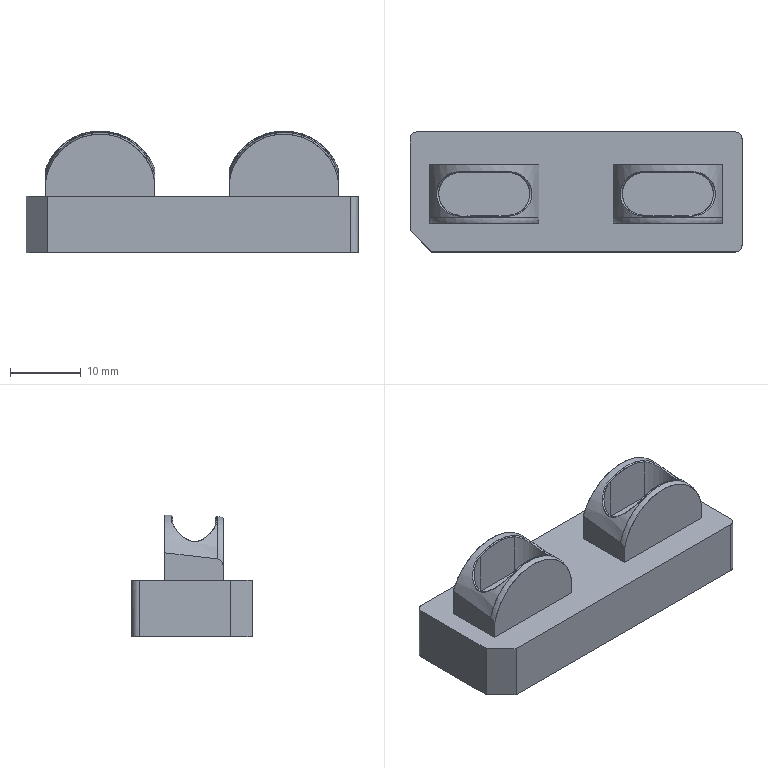NC program | PowerMill | posted with a generic post | part box 47 x 17 x 17.251 mm
Lines 1 to 1041 of 158620:
%
O0001
N104 ( POWERMILL CB  : 2026004.0)
N105 ( POST VER      : 2026.0.0.5161)
N106 ( OPTION FILE   : FANUC)
N107 ( OUTPUT WORKPLANE : WORLD)
N108 (  )
N109 ( TOOL LIST )
N110 (---------------------------------------)
N111 ( NO. | ID        | DIA.| TIP RAD|LENGTH)
N112 (---------------------------------------)
N113 (    1|D10C_1_1   |10.0 |  0.0   |72.72 )
N114 (   15|D3C_1_1    | 3.0 |  0.0   |64.44 )
N115 (    3|D10_1_1    |10.0 |  0.0   | 72.4 )
N116 (   22|R1.5_1_1   | 3.0 |  1.5   |63.12 )
N117 (   10|D3_1_1     | 3.0 |  0.0   |62.36 )
N118 (   13|TEXT_D4_1_1| 4.0 |  0.3   |64.52 )
N119 (---------------------------------------)
N120 (  )
N121 ( NUMBER OF TOOLPATHS: 11.0 )
N122 ( ESTIMATED PROGRAM DURATION: 0 HOURS 14 MIN 53 SEC)
N123 (  )
N124 G00 G21 G80 G40 G17
N125 G90
N126 G54
N127 G53 Z0.0
N128 (---------------)
N129 ( START TOOLPATH : 精公开粗01-扫面平行-D10C )
N130 (---------------)
N131 ( TOOL NO.    :1 )
N132 ( TOOL TYPE   : ENDMILL)
N133 ( TOOL ID     : D10C_1_1)
N134 ( TOOL DIA    : 10.0 LENGTH 72.72)
N135 T1
N136 M6
N137 S8000 M03
N138 G00 G90 X0.0 Y0.0
N139 G43 Z10.2 H1
N140
N141 G05 P10000 R4
N142 X31.28 Y11.28
N143 Z1.128
N144 G01 Z-0.072 F6000.0
N145 X26.28 F10000.0
N146 X-26.28
N147 Y5.64
N148 X26.28
N149 Y0.0
N150 X-26.28
N151 Y-5.64
N152 X26.28
N153 Y-11.28
N154 X-26.28
N155 X-31.28
N156 G00 Z10.2
N157 G05 P0
N158 (---------------)
N159 ( END TOOLPATH : 精公开粗01-扫面平行-D10C )
N160 (---------------)
N161 ( START TOOLPATH : 精公开粗01-外形偏置-D10C )
N162 (---------------)
N163 G00 X0.0 Y-0.283 Z9.878
N164 G05 P10000 R4
N165 X-17.5054 Y16.91
N166 Z0.6807
N167 G01 Z-0.5193 F6000.0
N168 Y16.3825 F10000.0
N169 G03 X-12.7579 Y11.635 I4.7475 J0.0
N170 G01 X12.758
N171 X12.7615 Y9.1322
N172 X15.0818 Y9.1355
N173 X15.8552 Y9.1085
N174 X16.5574 Y8.9981
N175 X17.4021 Y8.7405
N176 X18.1755 Y8.3597
N177 X18.393 Y8.2247
N178 X18.9489 Y7.8001
N179 X19.3124 Y7.4513
N180 X19.7224 Y6.9589
N181 X19.9196 Y6.6778
N182 X20.3286 Y5.9044
N183 X20.589 Y5.131
N184 X20.7229 Y4.3576
N185 X20.74 Y3.5841
N186 X20.657 Y2.8107
N187 X20.5342 Y2.0373
N188 X20.3467 Y1.2639
N189 X20.0249 Y0.4904
N190 X19.7224 Y-0.0237
N191 X19.5378 Y-0.283
N192 X19.22 Y-0.663
N193 G03 X19.1311 Y-1.2001 I0.3693 J-0.337
N194 G01 X19.4061 Y-1.8299
N195 X19.594 Y-2.6033
N196 X19.6618 Y-3.3767
N197 X19.6278 Y-4.1501
N198 X19.489 Y-4.9236
N199 X19.2244 Y-5.697
N200 X18.8199 Y-6.4704
N201 X18.2841 Y-7.2438
N202 X17.4821 Y-8.0173
N203 X16.6287 Y-8.6151
N204 X16.2904 Y-8.7907
N205 X15.8552 Y-8.9797
N206 X15.0818 Y-9.2292
N207 X14.3084 Y-9.4135
N208 X13.535 Y-9.5002
N209 X12.7615 Y-9.5116
N210 X11.9881 Y-9.4606
N211 X11.2147 Y-9.3047
N212 X10.4413 Y-9.0907
N213 X9.6678 Y-8.7734
N214 X8.8944 Y-8.3039
N215 X8.5171 Y-8.0173
N216 X8.121 Y-7.67
N217 X7.7159 Y-7.2438
N218 X7.3476 Y-6.7404
N219 X7.1809 Y-6.4704
N220 X6.7756 Y-5.697
N221 X6.5144 Y-4.9236
N222 X6.3722 Y-4.1501
N223 X6.3404 Y-3.3767
N224 X6.406 Y-2.6033
N225 X6.5939 Y-1.8299
N226 X6.8758 Y-1.1862
N227 G03 X6.7915 Y-0.6534 I-0.4579 J0.2006
N228 G01 X6.4622 Y-0.283
N229 X5.9751 Y0.4904
N230 X5.6533 Y1.2639
N231 X5.4678 Y2.0373
N232 X5.2617 Y3.5841
N233 X5.2771 Y4.3576
N234 X5.411 Y5.131
N235 X5.6731 Y5.9044
N236 X6.0812 Y6.6778
N237 X6.6856 Y7.4513
N238 X7.3476 Y8.0401
N239 X7.6061 Y8.2247
N240 X8.121 Y8.5254
N241 X8.8944 Y8.8474
N242 X9.4406 Y8.9981
N243 X10.4413 Y9.1289
N244 X12.7615 Y9.1322
N245 X12.758 Y11.635
N246 X27.507
N247 G02 X28.507 Y10.635 I0.0 J-1.0
N248 G01 Y-11.201
N249 G02 X27.507 Y-12.201 I-1.0 J0.0
N250 G01 X-27.507
N251 G02 X-28.507 Y-11.201 I0.0 J1.0
N252 G01 Y10.635
N253 G02 X-27.507 Y11.635 I1.0 J0.0
N254 G01 X-12.7579
N255 X-12.7615 Y9.1322
N256 X-10.4413 Y9.1288
N257 X-9.6678 Y9.0428
N258 X-8.8944 Y8.8473
N259 X-8.121 Y8.5254
N260 X-7.6061 Y8.2247
N261 X-7.3476 Y8.0401
N262 X-6.6856 Y7.4513
N263 X-6.0804 Y6.6778
N264 X-5.6713 Y5.9044
N265 X-5.411 Y5.131
N266 X-0.0017 Y6.1258
N267 X-0.0034 Y6.135
N268 X0.0034
N269 X0.0 Y6.1165
N270 X-0.0017 Y6.1258
N271 X-5.411 Y5.131
N272 X-5.2771 Y4.3576
N273 X-5.2608 Y3.5841
N274 X-5.3417 Y2.8107
N275 X-5.4657 Y2.0373
N276 X-5.6533 Y1.2639
N277 X-5.9751 Y0.4904
N278 X-6.4622 Y-0.283
N279 X-6.7824 Y-0.6429
N280 G03 X-6.8707 Y-1.1667 I0.3736 J-0.3323
N281 G01 X-6.5959 Y-1.8299
N282 X-6.406 Y-2.6033
N283 X-6.3433 Y-3.3392
N284 X-1.2755 Y-3.4159
N285 X-1.2507 Y-1.7746
N286 G02 X1.2556 Y-1.7764 I1.2532 J-0.019
N287 G01 X1.2811 Y-3.6293
N288 X1.3082 Y-4.2623
N289 X1.372 Y-4.8926
N290 X1.4318 Y-5.3509
N291 G02 X0.2456 Y-6.7289 I-1.2099 J-0.158
N292 G01 X-0.1982 Y-6.7375
N293 G02 X-1.431 Y-5.3585 I-0.0237 J1.2194
N294 G01 X-1.3708 Y-4.9021
N295 X-1.3067 Y-4.2776
N296 X-1.279 Y-3.6503
N297 X-1.2755 Y-3.4159
N298 X-6.3433 Y-3.3392
N299 X-6.3401 Y-3.3767
N300 X-6.3722 Y-4.1501
N301 X-6.5114 Y-4.9236
N302 X-6.7756 Y-5.697
N303 X-7.3476 Y-6.7404
N304 X-7.7213 Y-7.2438
N305 X-8.121 Y-7.67
N306 X-8.5201 Y-8.0173
N307 X-8.8944 Y-8.3039
N308 X-9.7111 Y-8.7907
N309 X-10.4413 Y-9.0907
N310 X-11.2147 Y-9.307
N311 X-11.9881 Y-9.4606
N312 X-12.7615 Y-9.5073
N313 X-13.535 Y-9.5014
N314 X-14.3084 Y-9.4135
N315 X-15.0818 Y-9.2292
N316 X-15.8552 Y-8.9797
N317 X-16.6287 Y-8.6151
N318 X-17.4813 Y-8.0173
N319 X-18.2841 Y-7.2438
N320 X-18.8183 Y-6.4704
N321 X-19.2244 Y-5.697
N322 X-19.4849 Y-4.9236
N323 X-19.6278 Y-4.1501
N324 X-19.6618 Y-3.3767
N325 X-19.594 Y-2.6033
N326 X-19.4061 Y-1.8299
N327 X-19.1308 Y-1.2012
N328 G03 X-19.2193 Y-0.6637 I-0.4579 J0.2006
N329 G01 X-19.7224 Y-0.0237
N330 X-20.0249 Y0.4904
N331 X-20.3467 Y1.2639
N332 X-20.4958 Y1.836
N333 X-20.7387 Y3.5841
N334 X-20.7229 Y4.3576
N335 X-20.5886 Y5.131
N336 X-20.3287 Y5.9044
N337 X-19.9196 Y6.6778
N338 X-19.7224 Y6.9585
N339 X-19.3142 Y7.4513
N340 X-18.9489 Y7.8001
N341 X-18.3932 Y8.2247
N342 X-18.1755 Y8.3596
N343 X-17.4021 Y8.7406
N344 X-16.6287 Y8.9813
N345 X-15.8552 Y9.1076
N346 X-15.0818 Y9.1355
N347 X-12.7615 Y9.1322
N348 X-12.7579 Y11.635
N349 G00 Z3.2834
N350 G01 X-17.5054 Y16.91
N351 G00 Z0.2834
N352 G01 Z-0.9166 F6000.0
N353 Y16.3825 F10000.0
N354 G03 X-12.7579 Y11.635 I4.7475 J0.0
N355 G01 X12.7615
N356 Y9.1356
N357 X15.8552
N358 X16.6287 Y9.1286
N359 X17.4021 Y9.0388
N360 X18.1755 Y8.8346
N361 X18.9489 Y8.4994
N362 X19.4118 Y8.2247
N363 X19.7224 Y7.9996
N364 X20.3275 Y7.4513
N365 X20.4958 Y7.2629
N366 X20.9306 Y6.6778
N367 X21.2692 Y6.053
N368 X21.598 Y5.131
N369 X21.7316 Y4.3576
N370 X21.7486 Y3.5841
N371 X21.6031 Y2.0373
N372 X21.4153 Y1.2639
N373 X21.2692 Y0.8725
N374 X21.0944 Y0.4904
N375 X20.6089 Y-0.283
N376 X20.5103 Y-0.4012
N377 G03 X20.4588 Y-0.9675 I0.3838 J-0.3204
N378 G01 X20.509 Y-1.0564
N379 X20.8302 Y-1.8299
N380 X21.0174 Y-2.6033
N381 X21.0885 Y-3.3767
N382 X21.0627 Y-4.1501
N383 X20.9277 Y-4.9236
N384 X20.6786 Y-5.697
N385 X20.3215 Y-6.4704
N386 X19.7224 Y-7.3692
N387 X18.9489 Y-8.1895
N388 X18.1887 Y-8.7907
N389 X17.4021 Y-9.2212
N390 X16.6287 Y-9.495
N391 X16.3488 Y-9.5641
N392 X15.8552 Y-9.6494
N393 X15.0818 Y-9.7019
N394 X11.2147 Y-9.702
N395 X10.4413 Y-9.6799
N396 X9.6501 Y-9.5641
N397 X8.8944 Y-9.3411
N398 X8.121 Y-8.9802
N399 X7.8138 Y-8.7907
N400 X7.3476 Y-8.4482
N401 X6.5741 Y-7.7184
N402 X6.1816 Y-7.2438
N403 X5.6785 Y-6.4704
N404 X5.3209 Y-5.697
N405 X5.0726 Y-4.9236
N406 X4.9365 Y-4.1501
N407 X4.9139 Y-3.3767
N408 X4.9804 Y-2.6274
N409 X0.4981 Y-2.2296
N410 X4.9804 Y-2.6274
N411 X4.9826 Y-2.6033
N412 X5.1699 Y-1.8299
N413 X5.491 Y-1.0564
N414 X5.5409 Y-0.9685
N415 G03 X5.4902 Y-0.4016 I-0.4348 J0.2468
N416 G01 X5.3913 Y-0.283
N417 X4.9056 Y0.4904
N418 X4.5841 Y1.2639
N419 X4.3969 Y2.0373
N420 X4.2538 Y3.5548
N421 Y4.166
N422 X4.4022 Y5.131
N423 X4.6628 Y5.9044
N424 X5.0273 Y6.6094
N425 X5.6719 Y7.4513
N426 X6.5741 Y8.2158
N427 X7.3476 Y8.6461
N428 X8.121 Y8.928
N429 X8.8944 Y9.0866
N430 X9.6678 Y9.1356
N431 X12.7615
N432 Y11.635
N433 X27.507
N434 G02 X28.507 Y10.635 I0.0 J-1.0
N435 G01 Y-11.201
N436 G02 X27.507 Y-12.201 I-1.0 J0.0
N437 G01 X-27.507
N438 G02 X-28.507 Y-11.201 I0.0 J1.0
N439 G01 Y10.635
N440 G02 X-27.507 Y11.635 I1.0 J0.0
N441 G01 X-12.7616
N442 X-12.7615 Y9.1356
N443 X-9.6678
N444 X-8.8944 Y9.0868
N445 X-8.121 Y8.928
N446 X-7.3476 Y8.6461
N447 X-6.5883 Y8.2247
N448 X-5.6719 Y7.4513
N449 X-5.0701 Y6.6778
N450 X-4.6616 Y5.9044
N451 X-4.402 Y5.131
N452 X-4.2684 Y4.3576
N453 X-4.2528 Y3.5841
N454 X-4.3974 Y2.0373
N455 X-4.5844 Y1.2639
N456 X-4.9053 Y0.4904
N457 X-5.3911 Y-0.283
N458 X-5.4897 Y-0.4012
N459 G03 X-5.5413 Y-0.9673 I0.3838 J-0.3203
N460 G01 X-5.491 Y-1.0564
N461 X-5.1698 Y-1.8299
N462 X-4.9826 Y-2.6033
N463 X-4.9133 Y-3.3767
N464 X-4.9373 Y-4.1501
N465 X-0.4941 Y-4.8628
N466 X-4.9373 Y-4.1501
N467 X-5.0723 Y-4.9236
N468 X-5.3222 Y-5.697
N469 X-5.6785 Y-6.4704
N470 X-6.1816 Y-7.2438
N471 X-6.5741 Y-7.7194
N472 X-6.8664 Y-8.0173
N473 X-7.3476 Y-8.4482
N474 X-7.8088 Y-8.7907
N475 X-8.121 Y-8.9802
N476 X-8.8944 Y-9.3411
N477 X-9.6512 Y-9.5641
N478 X-10.4413 Y-9.6799
N479 X-11.2147 Y-9.702
N480 X-15.0818 Y-9.7019
N481 X-15.8552 Y-9.6494
N482 X-16.6287 Y-9.495
N483 X-17.4021 Y-9.2212
N484 X-18.1925 Y-8.7907
N485 X-18.9489 Y-8.1895
N486 X-19.7224 Y-7.3692
N487 X-20.3215 Y-6.4704
N488 X-20.6791 Y-5.697
N489 X-20.9274 Y-4.9236
N490 X-21.0642 Y-4.1501
N491 X-21.089 Y-3.3767
N492 X-21.0174 Y-2.6033
N493 X-20.8302 Y-1.8299
N494 X-20.4958 Y-1.0376
N495 X-20.4566 Y-0.9678
N496 G03 X-20.5089 Y-0.4028 I-0.4361 J0.2446
N497 G01 X-20.6089 Y-0.283
N498 X-21.0947 Y0.4904
N499 X-21.4159 Y1.2639
N500 X-21.6027 Y2.0373
N501 X-21.7473 Y3.5841
N502 X-21.7315 Y4.3576
N503 X-21.5953 Y5.131
N504 X-21.3384 Y5.9044
N505 X-20.9307 Y6.6778
N506 X-20.4958 Y7.2621
N507 X-20.3242 Y7.4513
N508 X-19.7224 Y8.0
N509 X-19.4105 Y8.2247
N510 X-18.9489 Y8.4993
N511 X-18.1755 Y8.8344
N512 X-17.6027 Y8.9981
N513 X-16.6287 Y9.1293
N514 X-15.8552 Y9.1355
N515 X-12.7615 Y9.1356
N516 X-12.7616 Y11.635
N517 X-12.7579
N518 G00 Z2.8861
N519 G01 X-17.5054 Y16.91
N520 G00 Z-0.1139
N521 G01 Z-1.3139 F6000.0
N522 Y16.3825 F10000.0
N523 G03 X-12.7579 Y11.635 I4.7475 J0.0
N524 G01 X12.7615
N525 Y9.1356
N526 X16.6287
N527 X17.4021 Y9.1287
N528 X18.1755 Y9.0372
N529 X18.9489 Y8.8289
N530 X19.7224 Y8.4866
N531 X20.1585 Y8.2247
N532 X20.4958 Y7.9787
N533 X21.0707 Y7.4513
N534 X21.2692 Y7.2266
N535 X21.6726 Y6.6778
N536 X22.0427 Y5.9878
N537 X22.3387 Y5.131
N538 X22.4729 Y4.3576
N539 X22.4911 Y3.5841
N540 X22.3706 Y2.0373
N541 X22.1963 Y1.2639
N542 X22.0427 Y0.8274
N543 X21.8935 Y0.4904
N544 X21.4318 Y-0.283
N545 X21.3709 Y-0.3608
N546 G03 X21.3295 Y-0.9149 I0.3938 J-0.308
N547 G01 X21.4095 Y-1.0564
N548 X21.7259 Y-1.8299
N549 X21.9101 Y-2.6033
N550 X21.9743 Y-3.3767
N551 X21.94 Y-4.1501
N552 X21.8071 Y-4.9236
N553 X21.5882 Y-5.697
N554 X21.2692 Y-6.4134
N555 X20.7685 Y-7.2438
N556 X20.1242 Y-8.0173
N557 X19.7224 Y-8.3975
N558 X19.2077 Y-8.7907
N559 X18.9489 Y-8.9496
N560 X18.1755 Y-9.3259
N561 X17.3982 Y-9.5641
N562 X16.6287 Y-9.682
N563 X15.8552 Y-9.702
N564 X15.0872 Y-9.7015
N565 X15.0818 Y-9.7019
N566 X11.2147
N567 X11.1199 Y-9.6992
N568 X9.6678 Y-9.6984
N569 X8.8944 Y-9.6208
N570 X8.121 Y-9.4321
N571 X7.3476 Y-9.1118
N572 X6.7915 Y-8.7907
N573 X6.5741 Y-8.6344
N574 X5.8748 Y-8.0173
N575 X5.2294 Y-7.2438
N576 X4.7597 Y-6.4704
N577 X4.4109 Y-5.697
N578 X4.2538 Y-5.1845
N579 X4.0603 Y-4.1501
N580 X4.0257 Y-3.3767
N581 X4.0899 Y-2.6033
N582 X4.2538 Y-1.8981
N583 X4.59 Y-1.0564
N584 X4.671 Y-0.9135
N585 G03 X4.653 Y-0.3909 I-0.4349 J0.2466
N586 G01 X4.2538 Y0.2119
N587 X4.1071 Y0.4904
N588 X3.8058 Y1.2639
N589 X3.6321 Y2.0373
N590 X3.5092 Y3.5841
N591 X3.5274 Y4.3576
N592 X3.6609 Y5.131
N593 X3.9209 Y5.9044
N594 X4.2538 Y6.56
N595 X4.9289 Y7.4513
N596 X5.8007 Y8.1969
N597 X6.5741 Y8.6344
N598 X7.3476 Y8.9232
N599 X8.121 Y9.0853
N600 X8.8944 Y9.1356
N601 X12.7615
N602 Y11.635
N603 X27.507
N604 G02 X28.507 Y10.635 I0.0 J-1.0
N605 G01 Y-11.201
N606 G02 X27.507 Y-12.201 I-1.0 J0.0
N607 G01 X-27.507
N608 G02 X-28.507 Y-11.201 I0.0 J1.0
N609 G01 Y10.635
N610 G02 X-27.507 Y11.635 I1.0 J0.0
N611 G01 X-12.7615
N612 Y9.1356
N613 X-8.8944
N614 X-8.121 Y9.0853
N615 X-7.3476 Y8.9232
N616 X-6.5741 Y8.6362
N617 X-5.8419 Y8.2247
N618 X-5.0273 Y7.5531
N619 X-4.3261 Y6.6778
N620 X-3.9208 Y5.9044
N621 X-3.6605 Y5.131
N622 X-3.5273 Y4.3576
N623 X-3.5108 Y3.5841
N624 X-3.6293 Y2.0373
N625 X-3.8011 Y1.2639
N626 X-4.1055 Y0.4904
N627 X-4.2538 Y0.2074
N628 X-4.5686 Y-0.283
N629 X-4.6291 Y-0.3604
N630 G03 X-4.6704 Y-0.914 I0.3941 J-0.3078
N631 G01 X-4.59 Y-1.0564
N632 X-4.2744 Y-1.8299
N633 X-4.0913 Y-2.6033
N634 X-4.0265 Y-3.3767
N635 X-4.06 Y-4.1501
N636 X-4.1933 Y-4.9236
N637 X-4.4115 Y-5.697
N638 X-4.7597 Y-6.4704
N639 X-5.2294 Y-7.2438
N640 X-5.8007 Y-7.9322
N641 X-6.5741 Y-8.6344
N642 X-6.7931 Y-8.7907
N643 X-7.3476 Y-9.1118
N644 X-8.121 Y-9.4321
N645 X-8.5996 Y-9.5641
N646 X-8.8944 Y-9.6208
N647 X-9.6678 Y-9.6984
N648 X-11.1199 Y-9.6992
N649 X-11.2147 Y-9.7019
N650 X-15.0818
N651 X-15.0872 Y-9.7015
N652 X-15.8552 Y-9.702
N653 X-16.6287 Y-9.682
N654 X-17.4021 Y-9.562
N655 X-18.1755 Y-9.3259
N656 X-18.9489 Y-8.9496
N657 X-19.207 Y-8.7907
N658 X-19.7224 Y-8.3975
N659 X-20.1248 Y-8.0173
N660 X-20.7706 Y-7.2438
N661 X-21.2391 Y-6.4704
N662 X-21.5895 Y-5.697
N663 X-21.8073 Y-4.9236
N664 X-21.9376 Y-4.1501
N665 X-21.9742 Y-3.3767
N666 X-21.9101 Y-2.6033
N667 X-21.7267 Y-1.8299
N668 X-21.41 Y-1.0564
N669 X-21.3294 Y-0.9143
N670 G03 X-21.3702 Y-0.3601 I-0.435 J0.2466
N671 G01 X-21.4303 Y-0.283
N672 X-21.8919 Y0.4904
N673 X-22.0427 Y0.8315
N674 X-22.1963 Y1.2639
N675 X-22.3676 Y2.0373
N676 X-22.4911 Y3.5841
N677 X-22.4726 Y4.3576
N678 X-22.3405 Y5.131
N679 X-22.08 Y5.9044
N680 X-21.6727 Y6.6778
N681 X-21.2692 Y7.2266
N682 X-21.0702 Y7.4513
N683 X-20.4958 Y7.9789
N684 X-20.1595 Y8.2247
N685 X-19.7224 Y8.4861
N686 X-18.9489 Y8.8289
N687 X-18.362 Y8.9981
N688 X-17.4021 Y9.1291
N689 X-16.6287 Y9.1356
N690 X-12.7615
N691 Y11.635
N692 X-12.7579
N693 G00 Z2.4888
N694 G01 X-17.5054 Y16.91
N695 G00 Z-0.5112
N696 G01 Z-1.7112 F6000.0
N697 Y16.3825 F10000.0
N698 G03 X-12.7579 Y11.635 I4.7475 J0.0
N699 G01 X12.7615
N700 Y9.1356
N701 X16.6287
N702 X16.649 Y9.1354
N703 X17.4021 Y9.1356
N704 X18.1755 Y9.1176
N705 X18.9489 Y9.0023
N706 X19.7224 Y8.7661
N707 X20.4958 Y8.3906
N708 X20.7596 Y8.2247
N709 X21.2692 Y7.8358
N710 X21.6708 Y7.4513
N711 X22.0427 Y7.0073
N712 X22.2714 Y6.6778
N713 X22.6785 Y5.9044
N714 X22.8161 Y5.5434
N715 X22.9364 Y5.131
N716 X23.0704 Y4.3576
N717 X23.0861 Y3.5841
N718 X22.992 Y2.0373
N719 X22.8513 Y1.2639
N720 X22.5838 Y0.4904
N721 X22.1644 Y-0.283
N722 X22.1029 Y-0.37
N723 G03 X22.0689 Y-0.8923 I0.4081 J-0.2888
N724 G01 X22.1556 Y-1.0564
N725 X22.4497 Y-1.8299
N726 X22.6123 Y-2.6033
N727 X22.657 Y-3.3767
N728 X22.6102 Y-4.1501
N729 X22.4823 Y-4.9236
N730 X22.2652 Y-5.697
N731 X21.9441 Y-6.4704
N732 X21.4828 Y-7.2438
N733 X21.2692 Y-7.539
N734 X20.8699 Y-8.0173
N735 X20.4958 Y-8.3759
N736 X19.9578 Y-8.7907
N737 X19.7224 Y-8.9385
N738 X18.9489 Y-9.3192
N739 X18.1608 Y-9.5641
N740 X17.4021 Y-9.6818
N741 X16.6287 Y-9.702
N742 X15.867 Y-9.7016
N743 X15.8552 Y-9.7019
N744 X15.0872 Y-9.7015
N745 X15.0818 Y-9.7018
N746 X11.2147 Y-9.7019
N747 X11.1291 Y-9.6994
N748 X8.8944 Y-9.6984
N749 X8.121 Y-9.6205
N750 X7.3476 Y-9.4261
N751 X6.5741 Y-9.1025
N752 X6.0421 Y-8.7907
N753 X5.8007 Y-8.6181
N754 X5.1294 Y-8.0173
N755 X4.5173 Y-7.2438
N756 X4.2538 Y-6.8362
N757 X4.0562 Y-6.4704
N758 X3.7348 Y-5.697
N759 X3.5177 Y-4.9236
N760 X3.3891 Y-4.1501
N761 X3.3409 Y-3.3767
N762 X3.3864 Y-2.6033
N763 X3.55 Y-1.8299
N764 X3.8433 Y-1.0564
N765 X3.9306 Y-0.8921
N766 G03 X3.9214 Y-0.4064 I-0.4416 J0.2346
N767 G01 X3.4804 Y0.3529
N768 X3.1491 Y1.2639
N769 X3.0085 Y2.0373
N770 X2.9117 Y3.5841
N771 X2.9287 Y4.3576
N772 X3.062 Y5.131
N773 X3.3212 Y5.9044
N774 X3.4804 Y6.2424
N775 X3.7301 Y6.6778
N776 X4.2538 Y7.3686
N777 X5.0273 Y8.0723
N778 X5.24 Y8.2247
N779 X5.8007 Y8.5528
N780 X6.5741 Y8.8709
N781 X7.3476 Y9.0603
N782 X8.121 Y9.1335
N783 X8.8649 Y9.1337
N784 X8.8944 Y9.1356
N785 X12.7615
N786 Y11.635
N787 X27.507
N788 G02 X28.507 Y10.635 I0.0 J-1.0
N789 G01 Y-11.201
N790 G02 X27.507 Y-12.201 I-1.0 J0.0
N791 G01 X-27.507
N792 G02 X-28.507 Y-11.201 I0.0 J1.0
N793 G01 Y10.635
N794 G02 X-27.507 Y11.635 I1.0 J0.0
N795 G01 X-12.7615
N796 Y9.1356
N797 X-8.8944
N798 X-8.8651 Y9.1337
N799 X-8.121 Y9.1335
N800 X-7.3476 Y9.0603
N801 X-6.5741 Y8.8708
N802 X-5.8007 Y8.5528
N803 X-5.2408 Y8.2247
N804 X-5.0273 Y8.0736
N805 X-4.3299 Y7.4513
N806 X-3.7302 Y6.6778
N807 X-3.4804 Y6.2427
N808 X-3.3229 Y5.9044
N809 X-3.0629 Y5.131
N810 X-2.9298 Y4.3576
N811 X-2.9117 Y3.5841
N812 X-3.0085 Y2.0373
N813 X-3.149 Y1.2639
N814 X-3.4181 Y0.4904
N815 X-3.8364 Y-0.283
N816 X-3.8982 Y-0.3706
N817 G03 X-3.9325 Y-0.8908 I0.4086 J-0.2882
N818 G01 X-3.8458 Y-1.0564
N819 X-3.5503 Y-1.8299
N820 X-3.387 Y-2.6033
N821 X-3.3417 Y-3.3767
N822 X-3.3886 Y-4.1501
N823 X-3.4804 Y-4.73
N824 X-3.7348 Y-5.697
N825 X-4.0569 Y-6.4704
N826 X-4.2538 Y-6.8368
N827 X-4.5173 Y-7.2438
N828 X-5.0273 Y-7.9024
N829 X-5.8007 Y-8.6181
N830 X-6.0421 Y-8.7907
N831 X-6.5741 Y-9.1025
N832 X-7.3476 Y-9.4261
N833 X-7.8392 Y-9.5641
N834 X-8.121 Y-9.6205
N835 X-8.8944 Y-9.6984
N836 X-9.6678 Y-9.702
N837 X-16.6287
N838 X-17.4021 Y-9.6818
N839 X-18.1608 Y-9.5641
N840 X-18.9489 Y-9.3192
N841 X-19.7224 Y-8.9385
N842 X-19.9579 Y-8.7907
N843 X-20.4958 Y-8.3759
N844 X-20.8693 Y-8.0173
N845 X-21.2692 Y-7.539
N846 X-21.4827 Y-7.2438
N847 X-21.9441 Y-6.4704
N848 X-22.2652 Y-5.697
N849 X-22.4822 Y-4.9236
N850 X-22.6114 Y-4.1501
N851 X-22.6591 Y-3.3767
N852 X-22.611 Y-2.6033
N853 X-22.4502 Y-1.8299
N854 X-22.1568 Y-1.0564
N855 X-22.0702 Y-0.8935
N856 G03 X-22.1038 Y-0.3698 I-0.4415 J0.2346
N857 G01 X-22.1653 Y-0.283
N858 X-22.5824 Y0.4904
N859 X-22.8161 Y1.1388
N860 X-22.9914 Y2.0373
N861 X-23.0882 Y3.5841
N862 X-23.0713 Y4.3576
N863 X-22.9363 Y5.131
N864 X-22.8161 Y5.543
N865 X-22.6788 Y5.9044
N866 X-22.2718 Y6.6778
N867 X-22.0427 Y7.007
N868 X-21.6698 Y7.4513
N869 X-21.2692 Y7.8358
N870 X-20.7585 Y8.2247
N871 X-20.4958 Y8.3896
N872 X-19.7224 Y8.7658
N873 X-18.9674 Y8.9981
N874 X-18.1755 Y9.1176
N875 X-17.4021 Y9.1356
N876 X-16.6476 Y9.1354
N877 X-16.6287 Y9.1355
N878 X-12.7615 Y9.1356
N879 Y11.635
N880 X-12.7579
N881 G00 Z2.0915
N882 G01 X-17.5054 Y16.91
N883 G00 Z-0.9085
N884 G01 Z-2.1085 F6000.0
N885 Y16.3825 F10000.0
N886 G03 X-12.7579 Y11.635 I4.7475 J0.0
N887 G01 X27.507
N888 G02 X28.507 Y10.635 I0.0 J-1.0
N889 G01 Y-11.201
N890 G02 X27.507 Y-12.201 I-1.0 J0.0
N891 G01 X13.1483
N892 Y-9.702
N893 X8.8944
N894 X8.121 Y-9.6912
N895 X7.3476 Y-9.589
N896 X6.5741 Y-9.368
N897 X5.8007 Y-9.0111
N898 X5.4415 Y-8.7907
N899 X5.0273 Y-8.4806
N900 X4.5315 Y-8.0173
N901 X4.2538 Y-7.6938
N902 X3.9306 Y-7.2438
N903 X3.4867 Y-6.4704
N904 X3.1764 Y-5.697
N905 X2.9598 Y-4.9236
N906 X2.8417 Y-4.1501
N907 X2.7882 Y-3.3767
N908 X2.8012 Y-2.6033
N909 X2.9304 Y-1.8299
N910 X3.1824 Y-1.0564
N911 X3.2701 Y-0.8694
N912 G03 X3.2423 Y-0.3935 I-0.4526 J0.2123
N913 G01 X3.1738 Y-0.283
N914 X2.8114 Y0.4904
N915 X2.5901 Y1.2639
N916 X2.4891 Y2.0373
N917 X2.416 Y3.5841
N918 X2.4331 Y4.3576
N919 X2.5662 Y5.131
N920 X2.707 Y5.5995
N921 X2.8249 Y5.9044
N922 X3.2312 Y6.6778
N923 X3.4804 Y7.0336
N924 X3.8312 Y7.4513
N925 X4.2538 Y7.8555
N926 X4.7395 Y8.2247
N927 X5.0273 Y8.4049
N928 X5.8007 Y8.7767
N929 X6.5227 Y8.9981
N930 X7.3476 Y9.1218
N931 X8.121 Y9.1355
N932 X15.1107
N933 X16.6287
N934 X16.6291
N935 X18.1755
N936 X18.9489 Y9.0921
N937 X19.7224 Y8.935
N938 X20.4958 Y8.6522
N939 X21.2606 Y8.2247
N940 X22.0427 Y7.5796
N941 X22.169 Y7.4513
N942 X22.7688 Y6.6778
N943 X23.1751 Y5.9044
N944 X23.4339 Y5.131
N945 X23.567 Y4.3576
N946 X23.5895 Y3.8529
N947 X23.5118 Y2.0373
N948 X23.4105 Y1.2639
N949 X23.1879 Y0.4904
N950 X22.8161 Y-0.2979
N951 X22.7581 Y-0.3907
N952 G03 X22.7289 Y-0.8669 I0.424 J-0.265
N953 G01 X22.8172 Y-1.0564
N954 X23.072 Y-1.8299
N955 X23.2002 Y-2.6033
N956 X23.213 Y-3.3767
N957 X23.1588 Y-4.1501
N958 X23.0402 Y-4.9236
N959 X22.8236 Y-5.697
N960 X22.5129 Y-6.4704
N961 X22.0693 Y-7.2438
N962 X21.4688 Y-8.0173
N963 X21.2692 Y-8.2165
N964 X20.5586 Y-8.7907
N965 X19.7224 Y-9.2487
N966 X18.7703 Y-9.5641
N967 X18.1755 Y-9.6655
N968 X17.4021 Y-9.702
N969 X13.1483
N970 Y-12.201
N971 X-27.507
N972 G02 X-28.507 Y-11.201 I0.0 J1.0
N973 G01 Y10.635
N974 G02 X-27.507 Y11.635 I1.0 J0.0
N975 G01 X-13.1483
N976 Y9.1355
N977 X-8.121
N978 X-7.3476 Y9.1218
N979 X-6.5741 Y9.0087
N980 X-5.8007 Y8.7767
N981 X-5.0273 Y8.4045
N982 X-4.7394 Y8.2247
N983 X-4.2538 Y7.8539
N984 X-3.831 Y7.4513
N985 X-3.4804 Y7.0334
N986 X-3.2312 Y6.6778
N987 X-2.8249 Y5.9044
N988 X-2.5661 Y5.131
N989 X-2.433 Y4.3576
N990 X-2.4159 Y3.5841
N991 X-2.4885 Y2.0373
N992 X-2.5891 Y1.2639
N993 X-2.707 Y0.8013
N994 X-2.8128 Y0.4904
N995 X-3.175 Y-0.283
N996 X-3.2421 Y-0.3905
N997 G03 X-3.2707 Y-0.8672 I0.4242 J-0.2647
N998 G01 X-3.1821 Y-1.0564
N999 X-2.9285 Y-1.8299
N1000 X-2.8006 Y-2.6033
N1001 X-2.7874 Y-3.3767
N1002 X-2.8408 Y-4.1501
N1003 X-2.9598 Y-4.9236
N1004 X-3.1764 Y-5.697
N1005 X-3.4804 Y-6.4583
N1006 X-3.9306 Y-7.2438
N1007 X-4.2538 Y-7.6938
N1008 X-4.5313 Y-8.0173
N1009 X-5.0273 Y-8.4806
N1010 X-5.4416 Y-8.7907
N1011 X-5.8007 Y-9.0111
N1012 X-6.5741 Y-9.368
N1013 X-7.2304 Y-9.5641
N1014 X-8.121 Y-9.6912
N1015 X-8.8944 Y-9.702
N1016 X-17.4021
N1017 X-18.1755 Y-9.6655
N1018 X-18.7709 Y-9.5641
N1019 X-19.7224 Y-9.2487
N1020 X-20.4958 Y-8.8315
N1021 X-21.2692 Y-8.2165
N1022 X-21.4688 Y-8.0173
N1023 X-22.0427 Y-7.284
N1024 X-22.5131 Y-6.4704
N1025 X-22.8161 Y-5.7161
N1026 X-23.0402 Y-4.9236
N1027 X-23.1588 Y-4.1501
N1028 X-23.2126 Y-3.3767
N1029 X-23.1986 Y-2.6033
N1030 X-23.0699 Y-1.8299
N1031 X-22.8161 Y-1.0535
N1032 X-22.7297 Y-0.8692
N1033 G03 X-22.7577 Y-0.3931 I-0.4527 J0.2122
N1034 G01 X-22.8261 Y-0.283
N1035 X-23.1887 Y0.4904
N1036 X-23.4108 Y1.2639
N1037 X-23.509 Y2.0373
N1038 X-23.584 Y3.5841
N1039 X-23.5669 Y4.3576
N1040 X-23.4338 Y5.131
N1041 X-23.1749 Y5.9044
N1042 X-22.8161 Y6.5991
N1043 X-22.169 Y7.4513
N1044 X-22.0427 Y7.5802
N1045 X-21.2692 Y8.2179
N1046 X-20.4958 Y8.6525
N1047 X-19.7224 Y8.935
N1048 X-18.9489 Y9.0921
N1049 X-18.1755 Y9.1355
N1050 X-13.1483
N1051 Y11.635
N1052 X-12.7579
N1053 G00 Z1.6942
N1054 G01 X-17.5054 Y16.91
N1055 G00 Z-1.3058
N1056 G01 Z-2.5058 F6000.0
N1057 Y16.3825 F10000.0
N1058 G03 X-12.7579 Y11.635 I4.7475 J0.0
N1059 G01 X12.7615
N1060 Y9.1355
N1061 X18.1755
N1062 X18.9489 Y9.1293
N1063 X19.7224 Y9.0413
N1064 X20.4958 Y8.8337
N1065 X21.2692 Y8.4895
N1066 X21.708 Y8.2247
N1067 X22.0427 Y7.9803
N1068 X22.615 Y7.4513
N1069 X22.8161 Y7.2239
N1070 X23.2139 Y6.6778
N1071 X23.5895 Y5.9787
N1072 X23.8793 Y5.131
N1073 X24.012 Y4.3576
N1074 X24.0298 Y3.5841
N1075 X23.8904 Y1.2639
N1076 X23.7189 Y0.4904
N1077 X23.5895 Y0.1165
N1078 X23.4155 Y-0.283
N1079 X23.3448 Y-0.4172
N1080 G03 X23.3221 Y-0.8339 I0.4424 J-0.2331
N1081 G01 X23.41 Y-1.0564
N1082 X23.5895 Y-1.7053
N1083 X23.6976 Y-2.6033
N1084 X23.6283 Y-4.1501
N1085 X23.5153 Y-4.9236
N1086 X23.3021 Y-5.697
N1087 X22.9932 Y-6.4704
N1088 X22.5669 Y-7.2438
N1089 X22.0427 Y-7.9347
N1090 X21.2692 Y-8.6416
N1091 X21.059 Y-8.7907
N1092 X20.4958 Y-9.121
N1093 X19.7224 Y-9.4408
N1094 X19.2744 Y-9.5641
N1095 X18.9489 Y-9.6282
N1096 X18.1755 Y-9.7009
N1097 X17.423
N1098 X17.4021 Y-9.7019
N1099 X8.8944
N1100 X8.8917
N1101 X8.121 Y-9.702
N1102 X7.3476 Y-9.6688
N1103 X6.7243 Y-9.5641
N1104 X5.8007 Y-9.26
N1105 X5.0273 Y-8.8476
N1106 X4.2538 Y-8.24
N1107 X4.0326 Y-8.0173
N1108 X3.4804 Y-7.3164
N1109 X3.0066 Y-6.4704
N1110 X2.707 Y-5.7247
N1111 X2.4846 Y-4.9236
N1112 X2.3698 Y-4.1501
N1113 X2.3015 Y-2.6033
N1114 X2.3859 Y-1.8299
N1115 X2.5899 Y-1.0564
N1116 X2.6775 Y-0.8335
N1117 G03 X2.6542 Y-0.4168 I-0.4653 J0.183
N1118 G01 X2.5835 Y-0.283
N1119 X2.2819 Y0.4904
N1120 X2.1088 Y1.2639
N1121 X1.9706 Y3.5841
N1122 X1.989 Y4.3576
N1123 X2.122 Y5.131
N1124 X2.3796 Y5.9044
N1125 X2.707 Y6.5515
N1126 X3.3846 Y7.4513
N1127 X4.2538 Y8.1986
N1128 X5.0273 Y8.6401
N1129 X5.8007 Y8.9282
N1130 X6.5741 Y9.089
N1131 X7.3476 Y9.1356
N1132 X12.7615 Y9.1355
N1133 Y11.635
N1134 X27.507
N1135 G02 X28.507 Y10.635 I0.0 J-1.0
N1136 G01 Y-11.201
N1137 G02 X27.507 Y-12.201 I-1.0 J0.0
N1138 G01 X-27.507